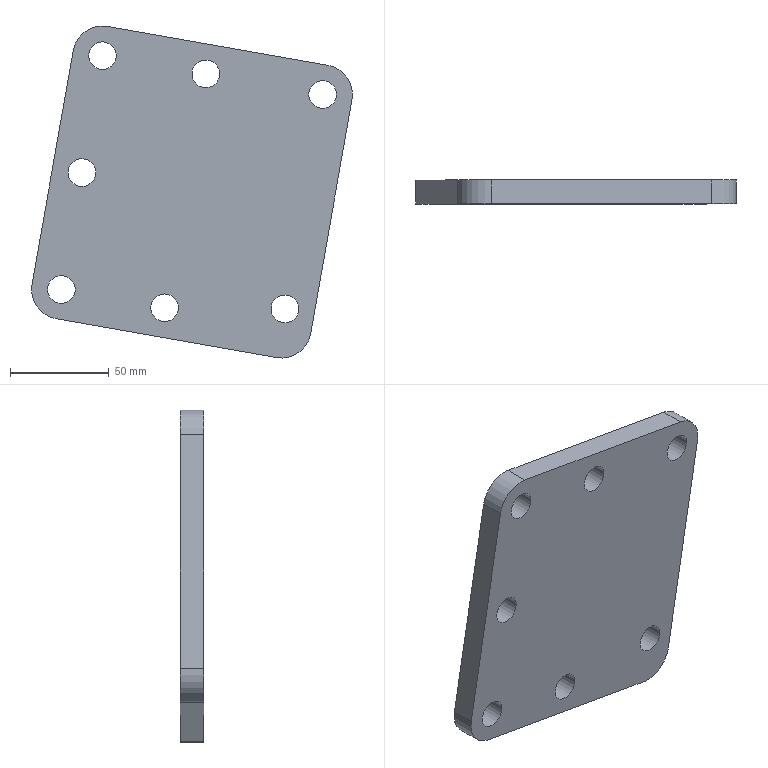Part | STEP file | front support mounting plate--000.001--20240925 | 1 solid | 17 faces | box 162.121 x 12 x 167.799 mm | volume 242152 mm3 | cylinder 11 | plane 6 | commonest cylinder face diameters 14 x7 30 x4
STEP:
#1=CARTESIAN_POINT('',(0.,0.,0.));
#2=DIRECTION('',(0.,0.,1.));
#3=DIRECTION('',(1.,0.,0.));
#4=AXIS2_PLACEMENT_3D('',#1,#2,#3);
#5=CARTESIAN_POINT('',(20.147,-188.5,-49.768));
#6=VERTEX_POINT('',#5);
#7=CARTESIAN_POINT('',(40.985,-188.5,68.409));
#8=VERTEX_POINT('',#7);
#9=CARTESIAN_POINT('',(11.873,-188.5,-96.689));
#10=DIRECTION('',(0.1736,0.,0.9848));
#11=VECTOR('',#10,1.);
#12=LINE('',#9,#11);
#13=CARTESIAN_POINT('',(30.566,-219.223,9.321));
#14=DIRECTION('',(0.9848,0.,-0.1736));
#15=DIRECTION('',(0.1736,0.,0.9848));
#16=AXIS2_PLACEMENT_3D('',#13,#14,#15);
#17=PLANE('',#16);
#18=CARTESIAN_POINT('',(-107.645,-30.723));
#19=DIRECTION('',(1.,0.));
#20=VECTOR('',#19,1.);
#21=LINE('',#18,#20);
#22=(GEOMETRIC_REPRESENTATION_CONTEXT(2)PARAMETRIC_REPRESENTATION_CONTEXT()REPRESENTATION_CONTEXT('',''));
#23=DEFINITIONAL_REPRESENTATION('',(#21),#22);
#24=PCURVE('',#17,#23);
#25=CARTESIAN_POINT('',(-243.192,-188.5,-51.714));
#26=DIRECTION('',(0.,-1.,0.));
#27=DIRECTION('',(0.1736,0.,0.9848));
#28=AXIS2_PLACEMENT_3D('',#25,#26,#27);
#29=PLANE('',#28);
#30=CARTESIAN_POINT('',(0.,-259.));
#31=DIRECTION('',(1.,0.));
#32=VECTOR('',#31,1.);
#33=LINE('',#30,#32);
#34=(GEOMETRIC_REPRESENTATION_CONTEXT(2)PARAMETRIC_REPRESENTATION_CONTEXT()REPRESENTATION_CONTEXT('',''));
#35=DEFINITIONAL_REPRESENTATION('',(#33),#34);
#36=PCURVE('',#29,#35);
#37=SURFACE_CURVE('',#12,(#24,#36),.PCURVE_S1.);
#38=EDGE_CURVE('',#6,#8,#37,.T.);
#39=ORIENTED_EDGE('',*,*,#38,.F.);
#40=CARTESIAN_POINT('',(20.147,-176.5,-49.768));
#41=VERTEX_POINT('',#40);
#42=CARTESIAN_POINT('',(20.147,-219.223,-49.768));
#43=DIRECTION('',(0.,1.,0.));
#44=VECTOR('',#43,1.);
#45=LINE('',#42,#44);
#46=CARTESIAN_POINT('',(-60.,0.));
#47=DIRECTION('',(0.,-1.));
#48=VECTOR('',#47,1.);
#49=LINE('',#46,#48);
#50=(GEOMETRIC_REPRESENTATION_CONTEXT(2)PARAMETRIC_REPRESENTATION_CONTEXT()REPRESENTATION_CONTEXT('',''));
#51=DEFINITIONAL_REPRESENTATION('',(#49),#50);
#52=PCURVE('',#17,#51);
#53=CARTESIAN_POINT('',(5.375,-188.5,-47.163));
#54=DIRECTION('',(0.,-1.,0.));
#55=DIRECTION('',(-0.2419,0.,-0.9703));
#56=AXIS2_PLACEMENT_3D('',#53,#54,#55);
#57=CYLINDRICAL_SURFACE('',#56,15.);
#58=CARTESIAN_POINT('',(1.641,30.723));
#59=DIRECTION('',(0.,-1.));
#60=VECTOR('',#59,1.);
#61=LINE('',#58,#60);
#62=(GEOMETRIC_REPRESENTATION_CONTEXT(2)PARAMETRIC_REPRESENTATION_CONTEXT()REPRESENTATION_CONTEXT('',''));
#63=DEFINITIONAL_REPRESENTATION('',(#61),#62);
#64=PCURVE('',#57,#63);
#65=SURFACE_CURVE('',#45,(#52,#64),.PCURVE_S1.);
#66=EDGE_CURVE('',#6,#41,#65,.T.);
#67=ORIENTED_EDGE('',*,*,#66,.T.);
#68=CARTESIAN_POINT('',(40.985,-176.5,68.409));
#69=VERTEX_POINT('',#68);
#70=CARTESIAN_POINT('',(11.873,-176.5,-96.689));
#71=DIRECTION('',(0.1736,0.,0.9848));
#72=VECTOR('',#71,1.);
#73=LINE('',#70,#72);
#74=CARTESIAN_POINT('',(-107.645,-42.723));
#75=DIRECTION('',(1.,0.));
#76=VECTOR('',#75,1.);
#77=LINE('',#74,#76);
#78=(GEOMETRIC_REPRESENTATION_CONTEXT(2)PARAMETRIC_REPRESENTATION_CONTEXT()REPRESENTATION_CONTEXT('',''));
#79=DEFINITIONAL_REPRESENTATION('',(#77),#78);
#80=PCURVE('',#17,#79);
#81=CARTESIAN_POINT('',(-243.192,-176.5,-51.714));
#82=DIRECTION('',(0.,-1.,0.));
#83=DIRECTION('',(0.1736,0.,0.9848));
#84=AXIS2_PLACEMENT_3D('',#81,#82,#83);
#85=PLANE('',#84);
#86=CARTESIAN_POINT('',(0.,-259.));
#87=DIRECTION('',(1.,0.));
#88=VECTOR('',#87,1.);
#89=LINE('',#86,#88);
#90=(GEOMETRIC_REPRESENTATION_CONTEXT(2)PARAMETRIC_REPRESENTATION_CONTEXT()REPRESENTATION_CONTEXT('',''));
#91=DEFINITIONAL_REPRESENTATION('',(#89),#90);
#92=PCURVE('',#85,#91);
#93=SURFACE_CURVE('',#73,(#80,#92),.PCURVE_S1.);
#94=EDGE_CURVE('',#41,#69,#93,.T.);
#95=ORIENTED_EDGE('',*,*,#94,.T.);
#96=CARTESIAN_POINT('',(40.985,-219.223,68.409));
#97=DIRECTION('',(0.,-1.,0.));
#98=VECTOR('',#97,1.);
#99=LINE('',#96,#98);
#100=CARTESIAN_POINT('',(60.,0.));
#101=DIRECTION('',(0.,1.));
#102=VECTOR('',#101,1.);
#103=LINE('',#100,#102);
#104=(GEOMETRIC_REPRESENTATION_CONTEXT(2)PARAMETRIC_REPRESENTATION_CONTEXT()REPRESENTATION_CONTEXT('',''));
#105=DEFINITIONAL_REPRESENTATION('',(#103),#104);
#106=PCURVE('',#17,#105);
#107=CARTESIAN_POINT('',(26.212,-188.5,71.014));
#108=DIRECTION('',(0.,1.,0.));
#109=DIRECTION('',(0.2419,0.,0.9703));
#110=AXIS2_PLACEMENT_3D('',#107,#108,#109);
#111=CYLINDRICAL_SURFACE('',#110,15.);
#112=CARTESIAN_POINT('',(1.501,-30.723));
#113=DIRECTION('',(0.,-1.));
#114=VECTOR('',#113,1.);
#115=LINE('',#112,#114);
#116=(GEOMETRIC_REPRESENTATION_CONTEXT(2)PARAMETRIC_REPRESENTATION_CONTEXT()REPRESENTATION_CONTEXT('',''));
#117=DEFINITIONAL_REPRESENTATION('',(#115),#116);
#118=PCURVE('',#111,#117);
#119=SURFACE_CURVE('',#99,(#106,#118),.PCURVE_S1.);
#120=EDGE_CURVE('',#69,#8,#119,.T.);
#121=ORIENTED_EDGE('',*,*,#120,.T.);
#122=EDGE_LOOP('',(#39,#67,#95,#121));
#123=FACE_BOUND('',#122,.T.);
#124=ADVANCED_FACE('',(#123),#17,.T.);
#125=CARTESIAN_POINT('',(28.817,-188.5,85.786));
#126=VERTEX_POINT('',#125);
#127=CARTESIAN_POINT('',(-82.466,-188.5,105.408));
#128=VERTEX_POINT('',#127);
#129=CARTESIAN_POINT('',(38.665,-188.5,84.049));
#130=DIRECTION('',(-0.9848,0.,0.1736));
#131=VECTOR('',#130,1.);
#132=LINE('',#129,#131);
#133=CARTESIAN_POINT('',(38.665,-188.5,84.049));
#134=DIRECTION('',(0.1736,0.,0.9848));
#135=DIRECTION('',(0.9848,0.,-0.1736));
#136=AXIS2_PLACEMENT_3D('',#133,#134,#135);
#137=PLANE('',#136);
#138=CARTESIAN_POINT('',(0.,0.));
#139=DIRECTION('',(-1.,0.));
#140=VECTOR('',#139,1.);
#141=LINE('',#138,#140);
#142=(GEOMETRIC_REPRESENTATION_CONTEXT(2)PARAMETRIC_REPRESENTATION_CONTEXT()REPRESENTATION_CONTEXT('',''));
#143=DEFINITIONAL_REPRESENTATION('',(#141),#142);
#144=PCURVE('',#137,#143);
#145=CARTESIAN_POINT('',(182.645,-254.));
#146=DIRECTION('',(0.,1.));
#147=VECTOR('',#146,1.);
#148=LINE('',#145,#147);
#149=(GEOMETRIC_REPRESENTATION_CONTEXT(2)PARAMETRIC_REPRESENTATION_CONTEXT()REPRESENTATION_CONTEXT('',''));
#150=DEFINITIONAL_REPRESENTATION('',(#148),#149);
#151=PCURVE('',#29,#150);
#152=SURFACE_CURVE('',#132,(#144,#151),.PCURVE_S1.);
#153=EDGE_CURVE('',#126,#128,#152,.T.);
#154=ORIENTED_EDGE('',*,*,#153,.F.);
#155=CARTESIAN_POINT('',(28.817,-176.5,85.786));
#156=VERTEX_POINT('',#155);
#157=CARTESIAN_POINT('',(28.817,-188.5,85.786));
#158=DIRECTION('',(0.,1.,0.));
#159=VECTOR('',#158,1.);
#160=LINE('',#157,#159);
#161=CARTESIAN_POINT('',(-10.,0.));
#162=DIRECTION('',(0.,1.));
#163=VECTOR('',#162,1.);
#164=LINE('',#161,#163);
#165=(GEOMETRIC_REPRESENTATION_CONTEXT(2)PARAMETRIC_REPRESENTATION_CONTEXT()REPRESENTATION_CONTEXT('',''));
#166=DEFINITIONAL_REPRESENTATION('',(#164),#165);
#167=PCURVE('',#137,#166);
#168=CARTESIAN_POINT('',(-0.06981,0.));
#169=DIRECTION('',(0.,1.));
#170=VECTOR('',#169,1.);
#171=LINE('',#168,#170);
#172=(GEOMETRIC_REPRESENTATION_CONTEXT(2)PARAMETRIC_REPRESENTATION_CONTEXT()REPRESENTATION_CONTEXT('',''));
#173=DEFINITIONAL_REPRESENTATION('',(#171),#172);
#174=PCURVE('',#111,#173);
#175=SURFACE_CURVE('',#160,(#167,#174),.PCURVE_S1.);
#176=EDGE_CURVE('',#126,#156,#175,.T.);
#177=ORIENTED_EDGE('',*,*,#176,.T.);
#178=CARTESIAN_POINT('',(-82.466,-176.5,105.408));
#179=VERTEX_POINT('',#178);
#180=CARTESIAN_POINT('',(-211.476,-176.5,128.156));
#181=DIRECTION('',(-0.9848,0.,0.1736));
#182=VECTOR('',#181,1.);
#183=LINE('',#180,#182);
#184=CARTESIAN_POINT('',(-254.,12.));
#185=DIRECTION('',(-1.,0.));
#186=VECTOR('',#185,1.);
#187=LINE('',#184,#186);
#188=(GEOMETRIC_REPRESENTATION_CONTEXT(2)PARAMETRIC_REPRESENTATION_CONTEXT()REPRESENTATION_CONTEXT('',''));
#189=DEFINITIONAL_REPRESENTATION('',(#187),#188);
#190=PCURVE('',#137,#189);
#191=CARTESIAN_POINT('',(182.645,0.));
#192=DIRECTION('',(0.,1.));
#193=VECTOR('',#192,1.);
#194=LINE('',#191,#193);
#195=(GEOMETRIC_REPRESENTATION_CONTEXT(2)PARAMETRIC_REPRESENTATION_CONTEXT()REPRESENTATION_CONTEXT('',''));
#196=DEFINITIONAL_REPRESENTATION('',(#194),#195);
#197=PCURVE('',#85,#196);
#198=SURFACE_CURVE('',#183,(#190,#197),.PCURVE_S1.);
#199=EDGE_CURVE('',#156,#179,#198,.T.);
#200=ORIENTED_EDGE('',*,*,#199,.T.);
#201=CARTESIAN_POINT('',(-82.466,-188.5,105.408));
#202=DIRECTION('',(0.,1.,0.));
#203=VECTOR('',#202,1.);
#204=LINE('',#201,#203);
#205=CARTESIAN_POINT('',(-123.,0.));
#206=DIRECTION('',(0.,1.));
#207=VECTOR('',#206,1.);
#208=LINE('',#205,#207);
#209=(GEOMETRIC_REPRESENTATION_CONTEXT(2)PARAMETRIC_REPRESENTATION_CONTEXT()REPRESENTATION_CONTEXT('',''));
#210=DEFINITIONAL_REPRESENTATION('',(#208),#209);
#211=PCURVE('',#137,#210);
#212=CARTESIAN_POINT('',(-85.071,-188.5,90.636));
#213=DIRECTION('',(0.,1.,0.));
#214=DIRECTION('',(0.2419,0.,0.9703));
#215=AXIS2_PLACEMENT_3D('',#212,#213,#214);
#216=CYLINDRICAL_SURFACE('',#215,15.);
#217=CARTESIAN_POINT('',(6.213,0.));
#218=DIRECTION('',(0.,1.));
#219=VECTOR('',#218,1.);
#220=LINE('',#217,#219);
#221=(GEOMETRIC_REPRESENTATION_CONTEXT(2)PARAMETRIC_REPRESENTATION_CONTEXT()REPRESENTATION_CONTEXT('',''));
#222=DEFINITIONAL_REPRESENTATION('',(#220),#221);
#223=PCURVE('',#216,#222);
#224=SURFACE_CURVE('',#204,(#211,#223),.PCURVE_S1.);
#225=EDGE_CURVE('',#128,#179,#224,.T.);
#226=ORIENTED_EDGE('',*,*,#225,.F.);
#227=EDGE_LOOP('',(#154,#177,#200,#226));
#228=FACE_BOUND('',#227,.T.);
#229=ADVANCED_FACE('',(#228),#137,.T.);
#230=CARTESIAN_POINT('',(-108.513,-176.5,-42.313));
#231=VERTEX_POINT('',#230);
#232=CARTESIAN_POINT('',(2.77,-176.5,-61.935));
#233=VERTEX_POINT('',#232);
#234=CARTESIAN_POINT('',(-237.523,-176.5,-19.565));
#235=DIRECTION('',(0.9848,0.,-0.1736));
#236=VECTOR('',#235,1.);
#237=LINE('',#234,#236);
#238=CARTESIAN_POINT('',(-108.513,-188.5,-42.313));
#239=DIRECTION('',(-0.1736,0.,-0.9848));
#240=DIRECTION('',(-0.9848,0.,0.1736));
#241=AXIS2_PLACEMENT_3D('',#238,#239,#240);
#242=PLANE('',#241);
#243=CARTESIAN_POINT('',(131.,12.));
#244=DIRECTION('',(-1.,0.));
#245=VECTOR('',#244,1.);
#246=LINE('',#243,#245);
#247=(GEOMETRIC_REPRESENTATION_CONTEXT(2)PARAMETRIC_REPRESENTATION_CONTEXT()REPRESENTATION_CONTEXT('',''));
#248=DEFINITIONAL_REPRESENTATION('',(#246),#247);
#249=PCURVE('',#242,#248);
#250=CARTESIAN_POINT('',(32.645,0.));
#251=DIRECTION('',(0.,-1.));
#252=VECTOR('',#251,1.);
#253=LINE('',#250,#252);
#254=(GEOMETRIC_REPRESENTATION_CONTEXT(2)PARAMETRIC_REPRESENTATION_CONTEXT()REPRESENTATION_CONTEXT('',''));
#255=DEFINITIONAL_REPRESENTATION('',(#253),#254);
#256=PCURVE('',#85,#255);
#257=SURFACE_CURVE('',#237,(#249,#256),.PCURVE_S1.);
#258=EDGE_CURVE('',#231,#233,#257,.T.);
#259=ORIENTED_EDGE('',*,*,#258,.T.);
#260=CARTESIAN_POINT('',(2.77,-188.5,-61.935));
#261=VERTEX_POINT('',#260);
#262=CARTESIAN_POINT('',(2.77,-188.5,-61.935));
#263=DIRECTION('',(0.,-1.,0.));
#264=VECTOR('',#263,1.);
#265=LINE('',#262,#264);
#266=CARTESIAN_POINT('',(-113.,0.));
#267=DIRECTION('',(0.,-1.));
#268=VECTOR('',#267,1.);
#269=LINE('',#266,#268);
#270=(GEOMETRIC_REPRESENTATION_CONTEXT(2)PARAMETRIC_REPRESENTATION_CONTEXT()REPRESENTATION_CONTEXT('',''));
#271=DEFINITIONAL_REPRESENTATION('',(#269),#270);
#272=PCURVE('',#242,#271);
#273=CARTESIAN_POINT('',(0.06981,0.));
#274=DIRECTION('',(0.,1.));
#275=VECTOR('',#274,1.);
#276=LINE('',#273,#275);
#277=(GEOMETRIC_REPRESENTATION_CONTEXT(2)PARAMETRIC_REPRESENTATION_CONTEXT()REPRESENTATION_CONTEXT('',''));
#278=DEFINITIONAL_REPRESENTATION('',(#276),#277);
#279=PCURVE('',#57,#278);
#280=SURFACE_CURVE('',#265,(#272,#279),.PCURVE_S1.);
#281=EDGE_CURVE('',#233,#261,#280,.T.);
#282=ORIENTED_EDGE('',*,*,#281,.T.);
#283=CARTESIAN_POINT('',(-108.513,-188.5,-42.313));
#284=VERTEX_POINT('',#283);
#285=CARTESIAN_POINT('',(-108.513,-188.5,-42.313));
#286=DIRECTION('',(0.9848,0.,-0.1736));
#287=VECTOR('',#286,1.);
#288=LINE('',#285,#287);
#289=CARTESIAN_POINT('',(0.,0.));
#290=DIRECTION('',(-1.,0.));
#291=VECTOR('',#290,1.);
#292=LINE('',#289,#291);
#293=(GEOMETRIC_REPRESENTATION_CONTEXT(2)PARAMETRIC_REPRESENTATION_CONTEXT()REPRESENTATION_CONTEXT('',''));
#294=DEFINITIONAL_REPRESENTATION('',(#292),#293);
#295=PCURVE('',#242,#294);
#296=CARTESIAN_POINT('',(32.645,-131.));
#297=DIRECTION('',(0.,-1.));
#298=VECTOR('',#297,1.);
#299=LINE('',#296,#298);
#300=(GEOMETRIC_REPRESENTATION_CONTEXT(2)PARAMETRIC_REPRESENTATION_CONTEXT()REPRESENTATION_CONTEXT('',''));
#301=DEFINITIONAL_REPRESENTATION('',(#299),#300);
#302=PCURVE('',#29,#301);
#303=SURFACE_CURVE('',#288,(#295,#302),.PCURVE_S1.);
#304=EDGE_CURVE('',#284,#261,#303,.T.);
#305=ORIENTED_EDGE('',*,*,#304,.F.);
#306=CARTESIAN_POINT('',(-108.513,-188.5,-42.313));
#307=DIRECTION('',(0.,1.,0.));
#308=VECTOR('',#307,1.);
#309=LINE('',#306,#308);
#310=CARTESIAN_POINT('',(0.,0.));
#311=DIRECTION('',(0.,1.));
#312=VECTOR('',#311,1.);
#313=LINE('',#310,#312);
#314=(GEOMETRIC_REPRESENTATION_CONTEXT(2)PARAMETRIC_REPRESENTATION_CONTEXT()REPRESENTATION_CONTEXT('',''));
#315=DEFINITIONAL_REPRESENTATION('',(#313),#314);
#316=PCURVE('',#242,#315);
#317=CARTESIAN_POINT('',(-105.909,-188.5,-27.541));
#318=DIRECTION('',(0.,1.,0.));
#319=DIRECTION('',(0.2419,0.,0.9703));
#320=AXIS2_PLACEMENT_3D('',#317,#318,#319);
#321=CYLINDRICAL_SURFACE('',#320,15.);
#322=CARTESIAN_POINT('',(3.072,0.));
#323=DIRECTION('',(0.,1.));
#324=VECTOR('',#323,1.);
#325=LINE('',#322,#324);
#326=(GEOMETRIC_REPRESENTATION_CONTEXT(2)PARAMETRIC_REPRESENTATION_CONTEXT()REPRESENTATION_CONTEXT('',''));
#327=DEFINITIONAL_REPRESENTATION('',(#325),#326);
#328=PCURVE('',#321,#327);
#329=SURFACE_CURVE('',#309,(#316,#328),.PCURVE_S1.);
#330=EDGE_CURVE('',#284,#231,#329,.T.);
#331=ORIENTED_EDGE('',*,*,#330,.T.);
#332=EDGE_LOOP('',(#259,#282,#305,#331));
#333=FACE_BOUND('',#332,.T.);
#334=ADVANCED_FACE('',(#333),#242,.T.);
#335=CARTESIAN_POINT('',(-83.377,-176.5,97.428));
#336=VERTEX_POINT('',#335);
#337=CARTESIAN_POINT('',(-85.071,-176.5,90.636));
#338=DIRECTION('',(0.,-1.,0.));
#339=DIRECTION('',(0.2419,0.,0.9703));
#340=AXIS2_PLACEMENT_3D('',#337,#338,#339);
#341=CIRCLE('',#340,7.);
#342=CARTESIAN_POINT('',(167.645,-131.));
#343=DIRECTION('',(0.9976,-0.06976));
#344=AXIS2_PLACEMENT_2D('',#342,#343);
#345=CIRCLE('',#344,7.);
#346=(GEOMETRIC_REPRESENTATION_CONTEXT(2)PARAMETRIC_REPRESENTATION_CONTEXT()REPRESENTATION_CONTEXT('',''));
#347=DEFINITIONAL_REPRESENTATION('',(#345),#346);
#348=PCURVE('',#85,#347);
#349=CARTESIAN_POINT('',(-85.071,-188.5,90.636));
#350=DIRECTION('',(0.,-1.,0.));
#351=DIRECTION('',(-0.2419,0.,-0.9703));
#352=AXIS2_PLACEMENT_3D('',#349,#350,#351);
#353=CYLINDRICAL_SURFACE('',#352,7.);
#354=CARTESIAN_POINT('',(3.142,-12.));
#355=DIRECTION('',(1.,0.));
#356=VECTOR('',#355,1.);
#357=LINE('',#354,#356);
#358=(GEOMETRIC_REPRESENTATION_CONTEXT(2)PARAMETRIC_REPRESENTATION_CONTEXT()REPRESENTATION_CONTEXT('',''));
#359=DEFINITIONAL_REPRESENTATION('',(#357),#358);
#360=PCURVE('',#353,#359);
#361=SURFACE_CURVE('',#341,(#348,#360),.PCURVE_S1.);
#362=EDGE_CURVE('',#336,#336,#361,.T.);
#363=ORIENTED_EDGE('',*,*,#362,.T.);
#364=EDGE_LOOP('',(#363));
#365=FACE_BOUND('',#364,.T.);
#366=CARTESIAN_POINT('',(-31.183,-176.5,88.225));
#367=VERTEX_POINT('',#366);
#368=CARTESIAN_POINT('',(-32.876,-176.5,81.433));
#369=DIRECTION('',(0.,-1.,0.));
#370=DIRECTION('',(0.2419,0.,0.9703));
#371=AXIS2_PLACEMENT_3D('',#368,#369,#370);
#372=CIRCLE('',#371,7.);
#373=CARTESIAN_POINT('',(167.645,-184.));
#374=DIRECTION('',(0.9976,-0.06976));
#375=AXIS2_PLACEMENT_2D('',#373,#374);
#376=CIRCLE('',#375,7.);
#377=(GEOMETRIC_REPRESENTATION_CONTEXT(2)PARAMETRIC_REPRESENTATION_CONTEXT()REPRESENTATION_CONTEXT('',''));
#378=DEFINITIONAL_REPRESENTATION('',(#376),#377);
#379=PCURVE('',#85,#378);
#380=CARTESIAN_POINT('',(-32.876,-188.5,81.433));
#381=DIRECTION('',(0.,-1.,0.));
#382=DIRECTION('',(-0.2419,0.,-0.9703));
#383=AXIS2_PLACEMENT_3D('',#380,#381,#382);
#384=CYLINDRICAL_SURFACE('',#383,7.);
#385=CARTESIAN_POINT('',(3.142,-12.));
#386=DIRECTION('',(1.,0.));
#387=VECTOR('',#386,1.);
#388=LINE('',#385,#387);
#389=(GEOMETRIC_REPRESENTATION_CONTEXT(2)PARAMETRIC_REPRESENTATION_CONTEXT()REPRESENTATION_CONTEXT('',''));
#390=DEFINITIONAL_REPRESENTATION('',(#388),#389);
#391=PCURVE('',#384,#390);
#392=SURFACE_CURVE('',#372,(#379,#391),.PCURVE_S1.);
#393=EDGE_CURVE('',#367,#367,#392,.T.);
#394=ORIENTED_EDGE('',*,*,#393,.T.);
#395=EDGE_LOOP('',(#394));
#396=FACE_BOUND('',#395,.T.);
#397=CARTESIAN_POINT('',(27.906,-176.5,77.806));
#398=VERTEX_POINT('',#397);
#399=CARTESIAN_POINT('',(26.212,-176.5,71.014));
#400=DIRECTION('',(0.,-1.,0.));
#401=DIRECTION('',(0.2419,0.,0.9703));
#402=AXIS2_PLACEMENT_3D('',#399,#400,#401);
#403=CIRCLE('',#402,7.);
#404=CARTESIAN_POINT('',(167.645,-244.));
#405=DIRECTION('',(0.9976,-0.06976));
#406=AXIS2_PLACEMENT_2D('',#404,#405);
#407=CIRCLE('',#406,7.);
#408=(GEOMETRIC_REPRESENTATION_CONTEXT(2)PARAMETRIC_REPRESENTATION_CONTEXT()REPRESENTATION_CONTEXT('',''));
#409=DEFINITIONAL_REPRESENTATION('',(#407),#408);
#410=PCURVE('',#85,#409);
#411=CARTESIAN_POINT('',(26.212,-188.5,71.014));
#412=DIRECTION('',(0.,-1.,0.));
#413=DIRECTION('',(-0.2419,0.,-0.9703));
#414=AXIS2_PLACEMENT_3D('',#411,#412,#413);
#415=CYLINDRICAL_SURFACE('',#414,7.);
#416=CARTESIAN_POINT('',(3.142,-12.));
#417=DIRECTION('',(1.,0.));
#418=VECTOR('',#417,1.);
#419=LINE('',#416,#418);
#420=(GEOMETRIC_REPRESENTATION_CONTEXT(2)PARAMETRIC_REPRESENTATION_CONTEXT()REPRESENTATION_CONTEXT('',''));
#421=DEFINITIONAL_REPRESENTATION('',(#419),#420);
#422=PCURVE('',#415,#421);
#423=SURFACE_CURVE('',#403,(#410,#422),.PCURVE_S1.);
#424=EDGE_CURVE('',#398,#398,#423,.T.);
#425=ORIENTED_EDGE('',*,*,#424,.T.);
#426=EDGE_LOOP('',(#425));
#427=FACE_BOUND('',#426,.T.);
#428=CARTESIAN_POINT('',(-93.796,-176.5,38.34));
#429=VERTEX_POINT('',#428);
#430=CARTESIAN_POINT('',(-95.49,-176.5,31.548));
#431=DIRECTION('',(0.,-1.,0.));
#432=DIRECTION('',(0.2419,0.,0.9703));
#433=AXIS2_PLACEMENT_3D('',#430,#431,#432);
#434=CIRCLE('',#433,7.);
#435=CARTESIAN_POINT('',(107.645,-131.));
#436=DIRECTION('',(0.9976,-0.06976));
#437=AXIS2_PLACEMENT_2D('',#435,#436);
#438=CIRCLE('',#437,7.);
#439=(GEOMETRIC_REPRESENTATION_CONTEXT(2)PARAMETRIC_REPRESENTATION_CONTEXT()REPRESENTATION_CONTEXT('',''));
#440=DEFINITIONAL_REPRESENTATION('',(#438),#439);
#441=PCURVE('',#85,#440);
#442=CARTESIAN_POINT('',(-95.49,-188.5,31.548));
#443=DIRECTION('',(0.,-1.,0.));
#444=DIRECTION('',(-0.2419,0.,-0.9703));
#445=AXIS2_PLACEMENT_3D('',#442,#443,#444);
#446=CYLINDRICAL_SURFACE('',#445,7.);
#447=CARTESIAN_POINT('',(3.142,-12.));
#448=DIRECTION('',(1.,0.));
#449=VECTOR('',#448,1.);
#450=LINE('',#447,#449);
#451=(GEOMETRIC_REPRESENTATION_CONTEXT(2)PARAMETRIC_REPRESENTATION_CONTEXT()REPRESENTATION_CONTEXT('',''));
#452=DEFINITIONAL_REPRESENTATION('',(#450),#451);
#453=PCURVE('',#446,#452);
#454=SURFACE_CURVE('',#434,(#441,#453),.PCURVE_S1.);
#455=EDGE_CURVE('',#429,#429,#454,.T.);
#456=ORIENTED_EDGE('',*,*,#455,.T.);
#457=EDGE_LOOP('',(#456));
#458=FACE_BOUND('',#457,.T.);
#459=CARTESIAN_POINT('',(8.805,-176.5,-30.523));
#460=VERTEX_POINT('',#459);
#461=CARTESIAN_POINT('',(7.111,-176.5,-37.315));
#462=DIRECTION('',(0.,-1.,0.));
#463=DIRECTION('',(0.2419,0.,0.9703));
#464=AXIS2_PLACEMENT_3D('',#461,#462,#463);
#465=CIRCLE('',#464,7.);
#466=CARTESIAN_POINT('',(57.645,-244.));
#467=DIRECTION('',(0.9976,-0.06976));
#468=AXIS2_PLACEMENT_2D('',#466,#467);
#469=CIRCLE('',#468,7.);
#470=(GEOMETRIC_REPRESENTATION_CONTEXT(2)PARAMETRIC_REPRESENTATION_CONTEXT()REPRESENTATION_CONTEXT('',''));
#471=DEFINITIONAL_REPRESENTATION('',(#469),#470);
#472=PCURVE('',#85,#471);
#473=CARTESIAN_POINT('',(7.111,-188.5,-37.315));
#474=DIRECTION('',(0.,-1.,0.));
#475=DIRECTION('',(-0.2419,0.,-0.9703));
#476=AXIS2_PLACEMENT_3D('',#473,#474,#475);
#477=CYLINDRICAL_SURFACE('',#476,7.);
#478=CARTESIAN_POINT('',(3.142,-12.));
#479=DIRECTION('',(1.,0.));
#480=VECTOR('',#479,1.);
#481=LINE('',#478,#480);
#482=(GEOMETRIC_REPRESENTATION_CONTEXT(2)PARAMETRIC_REPRESENTATION_CONTEXT()REPRESENTATION_CONTEXT('',''));
#483=DEFINITIONAL_REPRESENTATION('',(#481),#482);
#484=PCURVE('',#477,#483);
#485=SURFACE_CURVE('',#465,(#472,#484),.PCURVE_S1.);
#486=EDGE_CURVE('',#460,#460,#485,.T.);
#487=ORIENTED_EDGE('',*,*,#486,.T.);
#488=EDGE_LOOP('',(#487));
#489=FACE_BOUND('',#488,.T.);
#490=CARTESIAN_POINT('',(-104.215,-176.5,-20.749));
#491=VERTEX_POINT('',#490);
#492=CARTESIAN_POINT('',(-105.909,-176.5,-27.541));
#493=DIRECTION('',(0.,-1.,0.));
#494=DIRECTION('',(0.2419,0.,0.9703));
#495=AXIS2_PLACEMENT_3D('',#492,#493,#494);
#496=CIRCLE('',#495,7.);
#497=CARTESIAN_POINT('',(47.645,-131.));
#498=DIRECTION('',(0.9976,-0.06976));
#499=AXIS2_PLACEMENT_2D('',#497,#498);
#500=CIRCLE('',#499,7.);
#501=(GEOMETRIC_REPRESENTATION_CONTEXT(2)PARAMETRIC_REPRESENTATION_CONTEXT()REPRESENTATION_CONTEXT('',''));
#502=DEFINITIONAL_REPRESENTATION('',(#500),#501);
#503=PCURVE('',#85,#502);
#504=CARTESIAN_POINT('',(-105.909,-188.5,-27.541));
#505=DIRECTION('',(0.,-1.,0.));
#506=DIRECTION('',(-0.2419,0.,-0.9703));
#507=AXIS2_PLACEMENT_3D('',#504,#505,#506);
#508=CYLINDRICAL_SURFACE('',#507,7.);
#509=CARTESIAN_POINT('',(3.142,-12.));
#510=DIRECTION('',(1.,0.));
#511=VECTOR('',#510,1.);
#512=LINE('',#509,#511);
#513=(GEOMETRIC_REPRESENTATION_CONTEXT(2)PARAMETRIC_REPRESENTATION_CONTEXT()REPRESENTATION_CONTEXT('',''));
#514=DEFINITIONAL_REPRESENTATION('',(#512),#513);
#515=PCURVE('',#508,#514);
#516=SURFACE_CURVE('',#496,(#503,#515),.PCURVE_S1.);
#517=EDGE_CURVE('',#491,#491,#516,.T.);
#518=ORIENTED_EDGE('',*,*,#517,.T.);
#519=EDGE_LOOP('',(#518));
#520=FACE_BOUND('',#519,.T.);
#521=CARTESIAN_POINT('',(-52.02,-176.5,-29.952));
#522=VERTEX_POINT('',#521);
#523=CARTESIAN_POINT('',(-53.714,-176.5,-36.744));
#524=DIRECTION('',(0.,-1.,0.));
#525=DIRECTION('',(0.2419,0.,0.9703));
#526=AXIS2_PLACEMENT_3D('',#523,#524,#525);
#527=CIRCLE('',#526,7.);
#528=CARTESIAN_POINT('',(47.645,-184.));
#529=DIRECTION('',(0.9976,-0.06976));
#530=AXIS2_PLACEMENT_2D('',#528,#529);
#531=CIRCLE('',#530,7.);
#532=(GEOMETRIC_REPRESENTATION_CONTEXT(2)PARAMETRIC_REPRESENTATION_CONTEXT()REPRESENTATION_CONTEXT('',''));
#533=DEFINITIONAL_REPRESENTATION('',(#531),#532);
#534=PCURVE('',#85,#533);
#535=CARTESIAN_POINT('',(-53.714,-188.5,-36.744));
#536=DIRECTION('',(0.,-1.,0.));
#537=DIRECTION('',(-0.2419,0.,-0.9703));
#538=AXIS2_PLACEMENT_3D('',#535,#536,#537);
#539=CYLINDRICAL_SURFACE('',#538,7.);
#540=CARTESIAN_POINT('',(3.142,-12.));
#541=DIRECTION('',(1.,0.));
#542=VECTOR('',#541,1.);
#543=LINE('',#540,#542);
#544=(GEOMETRIC_REPRESENTATION_CONTEXT(2)PARAMETRIC_REPRESENTATION_CONTEXT()REPRESENTATION_CONTEXT('',''));
#545=DEFINITIONAL_REPRESENTATION('',(#543),#544);
#546=PCURVE('',#539,#545);
#547=SURFACE_CURVE('',#527,(#534,#546),.PCURVE_S1.);
#548=EDGE_CURVE('',#522,#522,#547,.T.);
#549=ORIENTED_EDGE('',*,*,#548,.T.);
#550=EDGE_LOOP('',(#549));
#551=FACE_BOUND('',#550,.T.);
#552=ORIENTED_EDGE('',*,*,#94,.F.);
#553=CARTESIAN_POINT('',(5.375,-176.5,-47.163));
#554=DIRECTION('',(0.,1.,0.));
#555=DIRECTION('',(0.2419,0.,0.9703));
#556=AXIS2_PLACEMENT_3D('',#553,#554,#555);
#557=CIRCLE('',#556,15.);
#558=CARTESIAN_POINT('',(62.608,-245.046));
#559=CARTESIAN_POINT('',(60.796,-270.964));
#560=CARTESIAN_POINT('',(39.257,-256.436));
#561=CARTESIAN_POINT('',(17.718,-241.907));
#562=CARTESIAN_POINT('',(41.069,-230.518));
#563=CARTESIAN_POINT('',(64.42,-219.129));
#564=CARTESIAN_POINT('',(62.608,-245.046));
#565=(BOUNDED_CURVE()B_SPLINE_CURVE(2,(#558,#559,#560,#561,#562,#563,#564),.UNSPECIFIED.,.T.,.F.)B_SPLINE_CURVE_WITH_KNOTS((1,2,2,2,2,1),(-2.094,0.,2.094,4.189,6.283,8.378),.UNSPECIFIED.)CURVE()GEOMETRIC_REPRESENTATION_ITEM()RATIONAL_B_SPLINE_CURVE((1.,0.5,1.,0.5,1.,0.5,1.))REPRESENTATION_ITEM(''));
#566=(GEOMETRIC_REPRESENTATION_CONTEXT(2)PARAMETRIC_REPRESENTATION_CONTEXT()REPRESENTATION_CONTEXT('',''));
#567=DEFINITIONAL_REPRESENTATION('',(#565),#566);
#568=PCURVE('',#85,#567);
#569=CARTESIAN_POINT('',(3.142,-12.));
#570=DIRECTION('',(-1.,0.));
#571=VECTOR('',#570,1.);
#572=LINE('',#569,#571);
#573=(GEOMETRIC_REPRESENTATION_CONTEXT(2)PARAMETRIC_REPRESENTATION_CONTEXT()REPRESENTATION_CONTEXT('',''));
#574=DEFINITIONAL_REPRESENTATION('',(#572),#573);
#575=PCURVE('',#57,#574);
#576=SURFACE_CURVE('',#557,(#568,#575),.PCURVE_S1.);
#577=EDGE_CURVE('',#41,#233,#576,.T.);
#578=ORIENTED_EDGE('',*,*,#577,.T.);
#579=ORIENTED_EDGE('',*,*,#258,.F.);
#580=CARTESIAN_POINT('',(-120.681,-176.5,-24.936));
#581=VERTEX_POINT('',#580);
#582=CARTESIAN_POINT('',(-105.909,-176.5,-27.541));
#583=DIRECTION('',(0.,1.,0.));
#584=DIRECTION('',(-0.2419,0.,-0.9703));
#585=AXIS2_PLACEMENT_3D('',#582,#583,#584);
#586=CIRCLE('',#585,15.);
#587=CARTESIAN_POINT('',(32.681,-129.954));
#588=CARTESIAN_POINT('',(34.494,-104.036));
#589=CARTESIAN_POINT('',(56.033,-118.564));
#590=CARTESIAN_POINT('',(77.572,-133.093));
#591=CARTESIAN_POINT('',(54.22,-144.482));
#592=CARTESIAN_POINT('',(30.869,-155.871));
#593=CARTESIAN_POINT('',(32.681,-129.954));
#594=(BOUNDED_CURVE()B_SPLINE_CURVE(2,(#587,#588,#589,#590,#591,#592,#593),.UNSPECIFIED.,.T.,.F.)B_SPLINE_CURVE_WITH_KNOTS((1,2,2,2,2,1),(-2.094,0.,2.094,4.189,6.283,8.378),.UNSPECIFIED.)CURVE()GEOMETRIC_REPRESENTATION_ITEM()RATIONAL_B_SPLINE_CURVE((1.,0.5,1.,0.5,1.,0.5,1.))REPRESENTATION_ITEM(''));
#595=(GEOMETRIC_REPRESENTATION_CONTEXT(2)PARAMETRIC_REPRESENTATION_CONTEXT()REPRESENTATION_CONTEXT('',''));
#596=DEFINITIONAL_REPRESENTATION('',(#594),#595);
#597=PCURVE('',#85,#596);
#598=CARTESIAN_POINT('',(-3.142,12.));
#599=DIRECTION('',(1.,0.));
#600=VECTOR('',#599,1.);
#601=LINE('',#598,#600);
#602=(GEOMETRIC_REPRESENTATION_CONTEXT(2)PARAMETRIC_REPRESENTATION_CONTEXT()REPRESENTATION_CONTEXT('',''));
#603=DEFINITIONAL_REPRESENTATION('',(#601),#602);
#604=PCURVE('',#321,#603);
#605=SURFACE_CURVE('',#586,(#597,#604),.PCURVE_S1.);
#606=EDGE_CURVE('',#231,#581,#605,.T.);
#607=ORIENTED_EDGE('',*,*,#606,.T.);
#608=CARTESIAN_POINT('',(-99.843,-176.5,93.241));
#609=VERTEX_POINT('',#608);
#610=CARTESIAN_POINT('',(-128.954,-176.5,-71.857));
#611=DIRECTION('',(-0.1736,0.,-0.9848));
#612=VECTOR('',#611,1.);
#613=LINE('',#610,#612);
#614=CARTESIAN_POINT('',(0.,-116.));
#615=DIRECTION('',(-1.,0.));
#616=VECTOR('',#615,1.);
#617=LINE('',#614,#616);
#618=(GEOMETRIC_REPRESENTATION_CONTEXT(2)PARAMETRIC_REPRESENTATION_CONTEXT()REPRESENTATION_CONTEXT('',''));
#619=DEFINITIONAL_REPRESENTATION('',(#617),#618);
#620=PCURVE('',#85,#619);
#621=CARTESIAN_POINT('',(-99.843,-188.5,93.241));
#622=DIRECTION('',(-0.9848,0.,0.1736));
#623=DIRECTION('',(0.1736,0.,0.9848));
#624=AXIS2_PLACEMENT_3D('',#621,#622,#623);
#625=PLANE('',#624);
#626=CARTESIAN_POINT('',(-167.645,12.));
#627=DIRECTION('',(-1.,0.));
#628=VECTOR('',#627,1.);
#629=LINE('',#626,#628);
#630=(GEOMETRIC_REPRESENTATION_CONTEXT(2)PARAMETRIC_REPRESENTATION_CONTEXT()REPRESENTATION_CONTEXT('',''));
#631=DEFINITIONAL_REPRESENTATION('',(#629),#630);
#632=PCURVE('',#625,#631);
#633=SURFACE_CURVE('',#613,(#620,#632),.PCURVE_S1.);
#634=EDGE_CURVE('',#609,#581,#633,.T.);
#635=ORIENTED_EDGE('',*,*,#634,.F.);
#636=CARTESIAN_POINT('',(-85.071,-176.5,90.636));
#637=DIRECTION('',(0.,1.,0.));
#638=DIRECTION('',(-0.2419,0.,-0.9703));
#639=AXIS2_PLACEMENT_3D('',#636,#637,#638);
#640=CIRCLE('',#639,15.);
#641=CARTESIAN_POINT('',(152.681,-129.954));
#642=CARTESIAN_POINT('',(154.494,-104.036));
#643=CARTESIAN_POINT('',(176.033,-118.564));
#644=CARTESIAN_POINT('',(197.572,-133.093));
#645=CARTESIAN_POINT('',(174.22,-144.482));
#646=CARTESIAN_POINT('',(150.869,-155.871));
#647=CARTESIAN_POINT('',(152.681,-129.954));
#648=(BOUNDED_CURVE()B_SPLINE_CURVE(2,(#641,#642,#643,#644,#645,#646,#647),.UNSPECIFIED.,.T.,.F.)B_SPLINE_CURVE_WITH_KNOTS((1,2,2,2,2,1),(-2.094,0.,2.094,4.189,6.283,8.378),.UNSPECIFIED.)CURVE()GEOMETRIC_REPRESENTATION_ITEM()RATIONAL_B_SPLINE_CURVE((1.,0.5,1.,0.5,1.,0.5,1.))REPRESENTATION_ITEM(''));
#649=(GEOMETRIC_REPRESENTATION_CONTEXT(2)PARAMETRIC_REPRESENTATION_CONTEXT()REPRESENTATION_CONTEXT('',''));
#650=DEFINITIONAL_REPRESENTATION('',(#648),#649);
#651=PCURVE('',#85,#650);
#652=CARTESIAN_POINT('',(3.142,12.));
#653=DIRECTION('',(1.,0.));
#654=VECTOR('',#653,1.);
#655=LINE('',#652,#654);
#656=(GEOMETRIC_REPRESENTATION_CONTEXT(2)PARAMETRIC_REPRESENTATION_CONTEXT()REPRESENTATION_CONTEXT('',''));
#657=DEFINITIONAL_REPRESENTATION('',(#655),#656);
#658=PCURVE('',#216,#657);
#659=SURFACE_CURVE('',#640,(#651,#658),.PCURVE_S1.);
#660=EDGE_CURVE('',#609,#179,#659,.T.);
#661=ORIENTED_EDGE('',*,*,#660,.T.);
#662=ORIENTED_EDGE('',*,*,#199,.F.);
#663=CARTESIAN_POINT('',(26.212,-176.5,71.014));
#664=DIRECTION('',(0.,1.,0.));
#665=DIRECTION('',(0.2419,0.,0.9703));
#666=AXIS2_PLACEMENT_3D('',#663,#664,#665);
#667=CIRCLE('',#666,15.);
#668=CARTESIAN_POINT('',(182.608,-245.046));
#669=CARTESIAN_POINT('',(180.796,-270.964));
#670=CARTESIAN_POINT('',(159.257,-256.436));
#671=CARTESIAN_POINT('',(137.718,-241.907));
#672=CARTESIAN_POINT('',(161.069,-230.518));
#673=CARTESIAN_POINT('',(184.42,-219.129));
#674=CARTESIAN_POINT('',(182.608,-245.046));
#675=(BOUNDED_CURVE()B_SPLINE_CURVE(2,(#668,#669,#670,#671,#672,#673,#674),.UNSPECIFIED.,.T.,.F.)B_SPLINE_CURVE_WITH_KNOTS((1,2,2,2,2,1),(-2.094,0.,2.094,4.189,6.283,8.378),.UNSPECIFIED.)CURVE()GEOMETRIC_REPRESENTATION_ITEM()RATIONAL_B_SPLINE_CURVE((1.,0.5,1.,0.5,1.,0.5,1.))REPRESENTATION_ITEM(''));
#676=(GEOMETRIC_REPRESENTATION_CONTEXT(2)PARAMETRIC_REPRESENTATION_CONTEXT()REPRESENTATION_CONTEXT('',''));
#677=DEFINITIONAL_REPRESENTATION('',(#675),#676);
#678=PCURVE('',#85,#677);
#679=CARTESIAN_POINT('',(-6.283,12.));
#680=DIRECTION('',(1.,0.));
#681=VECTOR('',#680,1.);
#682=LINE('',#679,#681);
#683=(GEOMETRIC_REPRESENTATION_CONTEXT(2)PARAMETRIC_REPRESENTATION_CONTEXT()REPRESENTATION_CONTEXT('',''));
#684=DEFINITIONAL_REPRESENTATION('',(#682),#683);
#685=PCURVE('',#111,#684);
#686=SURFACE_CURVE('',#667,(#678,#685),.PCURVE_S1.);
#687=EDGE_CURVE('',#156,#69,#686,.T.);
#688=ORIENTED_EDGE('',*,*,#687,.T.);
#689=EDGE_LOOP('',(#552,#578,#579,#607,#635,#661,#662,#688));
#690=FACE_BOUND('',#689,.T.);
#691=ADVANCED_FACE('',(#365,#396,#427,#458,#489,#520,#551,#690),#85,.F.);
#692=CARTESIAN_POINT('',(-52.02,-188.5,-29.952));
#693=VERTEX_POINT('',#692);
#694=CARTESIAN_POINT('',(-53.714,-188.5,-36.744));
#695=DIRECTION('',(0.,-1.,0.));
#696=DIRECTION('',(0.2419,0.,0.9703));
#697=AXIS2_PLACEMENT_3D('',#694,#695,#696);
#698=CIRCLE('',#697,7.);
#699=CARTESIAN_POINT('',(47.645,-184.));
#700=DIRECTION('',(0.9976,-0.06976));
#701=AXIS2_PLACEMENT_2D('',#699,#700);
#702=CIRCLE('',#701,7.);
#703=(GEOMETRIC_REPRESENTATION_CONTEXT(2)PARAMETRIC_REPRESENTATION_CONTEXT()REPRESENTATION_CONTEXT('',''));
#704=DEFINITIONAL_REPRESENTATION('',(#702),#703);
#705=PCURVE('',#29,#704);
#706=CARTESIAN_POINT('',(3.142,0.));
#707=DIRECTION('',(1.,0.));
#708=VECTOR('',#707,1.);
#709=LINE('',#706,#708);
#710=(GEOMETRIC_REPRESENTATION_CONTEXT(2)PARAMETRIC_REPRESENTATION_CONTEXT()REPRESENTATION_CONTEXT('',''));
#711=DEFINITIONAL_REPRESENTATION('',(#709),#710);
#712=PCURVE('',#539,#711);
#713=SURFACE_CURVE('',#698,(#705,#712),.PCURVE_S1.);
#714=EDGE_CURVE('',#693,#693,#713,.T.);
#715=ORIENTED_EDGE('',*,*,#714,.F.);
#716=EDGE_LOOP('',(#715));
#717=FACE_BOUND('',#716,.T.);
#718=CARTESIAN_POINT('',(-104.215,-188.5,-20.749));
#719=VERTEX_POINT('',#718);
#720=CARTESIAN_POINT('',(-105.909,-188.5,-27.541));
#721=DIRECTION('',(0.,-1.,0.));
#722=DIRECTION('',(0.2419,0.,0.9703));
#723=AXIS2_PLACEMENT_3D('',#720,#721,#722);
#724=CIRCLE('',#723,7.);
#725=CARTESIAN_POINT('',(47.645,-131.));
#726=DIRECTION('',(0.9976,-0.06976));
#727=AXIS2_PLACEMENT_2D('',#725,#726);
#728=CIRCLE('',#727,7.);
#729=(GEOMETRIC_REPRESENTATION_CONTEXT(2)PARAMETRIC_REPRESENTATION_CONTEXT()REPRESENTATION_CONTEXT('',''));
#730=DEFINITIONAL_REPRESENTATION('',(#728),#729);
#731=PCURVE('',#29,#730);
#732=CARTESIAN_POINT('',(3.142,0.));
#733=DIRECTION('',(1.,0.));
#734=VECTOR('',#733,1.);
#735=LINE('',#732,#734);
#736=(GEOMETRIC_REPRESENTATION_CONTEXT(2)PARAMETRIC_REPRESENTATION_CONTEXT()REPRESENTATION_CONTEXT('',''));
#737=DEFINITIONAL_REPRESENTATION('',(#735),#736);
#738=PCURVE('',#508,#737);
#739=SURFACE_CURVE('',#724,(#731,#738),.PCURVE_S1.);
#740=EDGE_CURVE('',#719,#719,#739,.T.);
#741=ORIENTED_EDGE('',*,*,#740,.F.);
#742=EDGE_LOOP('',(#741));
#743=FACE_BOUND('',#742,.T.);
#744=CARTESIAN_POINT('',(8.805,-188.5,-30.523));
#745=VERTEX_POINT('',#744);
#746=CARTESIAN_POINT('',(7.111,-188.5,-37.315));
#747=DIRECTION('',(0.,-1.,0.));
#748=DIRECTION('',(0.2419,0.,0.9703));
#749=AXIS2_PLACEMENT_3D('',#746,#747,#748);
#750=CIRCLE('',#749,7.);
#751=CARTESIAN_POINT('',(57.645,-244.));
#752=DIRECTION('',(0.9976,-0.06976));
#753=AXIS2_PLACEMENT_2D('',#751,#752);
#754=CIRCLE('',#753,7.);
#755=(GEOMETRIC_REPRESENTATION_CONTEXT(2)PARAMETRIC_REPRESENTATION_CONTEXT()REPRESENTATION_CONTEXT('',''));
#756=DEFINITIONAL_REPRESENTATION('',(#754),#755);
#757=PCURVE('',#29,#756);
#758=CARTESIAN_POINT('',(3.142,0.));
#759=DIRECTION('',(1.,0.));
#760=VECTOR('',#759,1.);
#761=LINE('',#758,#760);
#762=(GEOMETRIC_REPRESENTATION_CONTEXT(2)PARAMETRIC_REPRESENTATION_CONTEXT()REPRESENTATION_CONTEXT('',''));
#763=DEFINITIONAL_REPRESENTATION('',(#761),#762);
#764=PCURVE('',#477,#763);
#765=SURFACE_CURVE('',#750,(#757,#764),.PCURVE_S1.);
#766=EDGE_CURVE('',#745,#745,#765,.T.);
#767=ORIENTED_EDGE('',*,*,#766,.F.);
#768=EDGE_LOOP('',(#767));
#769=FACE_BOUND('',#768,.T.);
#770=CARTESIAN_POINT('',(-93.796,-188.5,38.34));
#771=VERTEX_POINT('',#770);
#772=CARTESIAN_POINT('',(-95.49,-188.5,31.548));
#773=DIRECTION('',(0.,-1.,0.));
#774=DIRECTION('',(0.2419,0.,0.9703));
#775=AXIS2_PLACEMENT_3D('',#772,#773,#774);
#776=CIRCLE('',#775,7.);
#777=CARTESIAN_POINT('',(107.645,-131.));
#778=DIRECTION('',(0.9976,-0.06976));
#779=AXIS2_PLACEMENT_2D('',#777,#778);
#780=CIRCLE('',#779,7.);
#781=(GEOMETRIC_REPRESENTATION_CONTEXT(2)PARAMETRIC_REPRESENTATION_CONTEXT()REPRESENTATION_CONTEXT('',''));
#782=DEFINITIONAL_REPRESENTATION('',(#780),#781);
#783=PCURVE('',#29,#782);
#784=CARTESIAN_POINT('',(3.142,0.));
#785=DIRECTION('',(1.,0.));
#786=VECTOR('',#785,1.);
#787=LINE('',#784,#786);
#788=(GEOMETRIC_REPRESENTATION_CONTEXT(2)PARAMETRIC_REPRESENTATION_CONTEXT()REPRESENTATION_CONTEXT('',''));
#789=DEFINITIONAL_REPRESENTATION('',(#787),#788);
#790=PCURVE('',#446,#789);
#791=SURFACE_CURVE('',#776,(#783,#790),.PCURVE_S1.);
#792=EDGE_CURVE('',#771,#771,#791,.T.);
#793=ORIENTED_EDGE('',*,*,#792,.F.);
#794=EDGE_LOOP('',(#793));
#795=FACE_BOUND('',#794,.T.);
#796=CARTESIAN_POINT('',(27.906,-188.5,77.806));
#797=VERTEX_POINT('',#796);
#798=CARTESIAN_POINT('',(26.212,-188.5,71.014));
#799=DIRECTION('',(0.,-1.,0.));
#800=DIRECTION('',(0.2419,0.,0.9703));
#801=AXIS2_PLACEMENT_3D('',#798,#799,#800);
#802=CIRCLE('',#801,7.);
#803=CARTESIAN_POINT('',(167.645,-244.));
#804=DIRECTION('',(0.9976,-0.06976));
#805=AXIS2_PLACEMENT_2D('',#803,#804);
#806=CIRCLE('',#805,7.);
#807=(GEOMETRIC_REPRESENTATION_CONTEXT(2)PARAMETRIC_REPRESENTATION_CONTEXT()REPRESENTATION_CONTEXT('',''));
#808=DEFINITIONAL_REPRESENTATION('',(#806),#807);
#809=PCURVE('',#29,#808);
#810=CARTESIAN_POINT('',(3.142,0.));
#811=DIRECTION('',(1.,0.));
#812=VECTOR('',#811,1.);
#813=LINE('',#810,#812);
#814=(GEOMETRIC_REPRESENTATION_CONTEXT(2)PARAMETRIC_REPRESENTATION_CONTEXT()REPRESENTATION_CONTEXT('',''));
#815=DEFINITIONAL_REPRESENTATION('',(#813),#814);
#816=PCURVE('',#415,#815);
#817=SURFACE_CURVE('',#802,(#809,#816),.PCURVE_S1.);
#818=EDGE_CURVE('',#797,#797,#817,.T.);
#819=ORIENTED_EDGE('',*,*,#818,.F.);
#820=EDGE_LOOP('',(#819));
#821=FACE_BOUND('',#820,.T.);
#822=CARTESIAN_POINT('',(-31.183,-188.5,88.225));
#823=VERTEX_POINT('',#822);
#824=CARTESIAN_POINT('',(-32.876,-188.5,81.433));
#825=DIRECTION('',(0.,-1.,0.));
#826=DIRECTION('',(0.2419,0.,0.9703));
#827=AXIS2_PLACEMENT_3D('',#824,#825,#826);
#828=CIRCLE('',#827,7.);
#829=CARTESIAN_POINT('',(167.645,-184.));
#830=DIRECTION('',(0.9976,-0.06976));
#831=AXIS2_PLACEMENT_2D('',#829,#830);
#832=CIRCLE('',#831,7.);
#833=(GEOMETRIC_REPRESENTATION_CONTEXT(2)PARAMETRIC_REPRESENTATION_CONTEXT()REPRESENTATION_CONTEXT('',''));
#834=DEFINITIONAL_REPRESENTATION('',(#832),#833);
#835=PCURVE('',#29,#834);
#836=CARTESIAN_POINT('',(3.142,0.));
#837=DIRECTION('',(1.,0.));
#838=VECTOR('',#837,1.);
#839=LINE('',#836,#838);
#840=(GEOMETRIC_REPRESENTATION_CONTEXT(2)PARAMETRIC_REPRESENTATION_CONTEXT()REPRESENTATION_CONTEXT('',''));
#841=DEFINITIONAL_REPRESENTATION('',(#839),#840);
#842=PCURVE('',#384,#841);
#843=SURFACE_CURVE('',#828,(#835,#842),.PCURVE_S1.);
#844=EDGE_CURVE('',#823,#823,#843,.T.);
#845=ORIENTED_EDGE('',*,*,#844,.F.);
#846=EDGE_LOOP('',(#845));
#847=FACE_BOUND('',#846,.T.);
#848=CARTESIAN_POINT('',(-83.377,-188.5,97.428));
#849=VERTEX_POINT('',#848);
#850=CARTESIAN_POINT('',(-85.071,-188.5,90.636));
#851=DIRECTION('',(0.,-1.,0.));
#852=DIRECTION('',(0.2419,0.,0.9703));
#853=AXIS2_PLACEMENT_3D('',#850,#851,#852);
#854=CIRCLE('',#853,7.);
#855=CARTESIAN_POINT('',(167.645,-131.));
#856=DIRECTION('',(0.9976,-0.06976));
#857=AXIS2_PLACEMENT_2D('',#855,#856);
#858=CIRCLE('',#857,7.);
#859=(GEOMETRIC_REPRESENTATION_CONTEXT(2)PARAMETRIC_REPRESENTATION_CONTEXT()REPRESENTATION_CONTEXT('',''));
#860=DEFINITIONAL_REPRESENTATION('',(#858),#859);
#861=PCURVE('',#29,#860);
#862=CARTESIAN_POINT('',(3.142,0.));
#863=DIRECTION('',(1.,0.));
#864=VECTOR('',#863,1.);
#865=LINE('',#862,#864);
#866=(GEOMETRIC_REPRESENTATION_CONTEXT(2)PARAMETRIC_REPRESENTATION_CONTEXT()REPRESENTATION_CONTEXT('',''));
#867=DEFINITIONAL_REPRESENTATION('',(#865),#866);
#868=PCURVE('',#353,#867);
#869=SURFACE_CURVE('',#854,(#861,#868),.PCURVE_S1.);
#870=EDGE_CURVE('',#849,#849,#869,.T.);
#871=ORIENTED_EDGE('',*,*,#870,.F.);
#872=EDGE_LOOP('',(#871));
#873=FACE_BOUND('',#872,.T.);
#874=ORIENTED_EDGE('',*,*,#304,.T.);
#875=CARTESIAN_POINT('',(5.375,-188.5,-47.163));
#876=DIRECTION('',(0.,-1.,0.));
#877=DIRECTION('',(0.2419,0.,0.9703));
#878=AXIS2_PLACEMENT_3D('',#875,#876,#877);
#879=CIRCLE('',#878,15.);
#880=CARTESIAN_POINT('',(47.645,-244.));
#881=DIRECTION('',(0.9976,-0.06976));
#882=AXIS2_PLACEMENT_2D('',#880,#881);
#883=CIRCLE('',#882,15.);
#884=(GEOMETRIC_REPRESENTATION_CONTEXT(2)PARAMETRIC_REPRESENTATION_CONTEXT()REPRESENTATION_CONTEXT('',''));
#885=DEFINITIONAL_REPRESENTATION('',(#883),#884);
#886=PCURVE('',#29,#885);
#887=CARTESIAN_POINT('',(-3.142,0.));
#888=DIRECTION('',(1.,0.));
#889=VECTOR('',#888,1.);
#890=LINE('',#887,#889);
#891=(GEOMETRIC_REPRESENTATION_CONTEXT(2)PARAMETRIC_REPRESENTATION_CONTEXT()REPRESENTATION_CONTEXT('',''));
#892=DEFINITIONAL_REPRESENTATION('',(#890),#891);
#893=PCURVE('',#57,#892);
#894=SURFACE_CURVE('',#879,(#886,#893),.PCURVE_S1.);
#895=EDGE_CURVE('',#261,#6,#894,.T.);
#896=ORIENTED_EDGE('',*,*,#895,.T.);
#897=ORIENTED_EDGE('',*,*,#38,.T.);
#898=CARTESIAN_POINT('',(26.212,-188.5,71.014));
#899=DIRECTION('',(0.,-1.,0.));
#900=DIRECTION('',(0.2419,0.,0.9703));
#901=AXIS2_PLACEMENT_3D('',#898,#899,#900);
#902=CIRCLE('',#901,15.);
#903=CARTESIAN_POINT('',(167.645,-244.));
#904=DIRECTION('',(0.9976,-0.06976));
#905=AXIS2_PLACEMENT_2D('',#903,#904);
#906=CIRCLE('',#905,15.);
#907=(GEOMETRIC_REPRESENTATION_CONTEXT(2)PARAMETRIC_REPRESENTATION_CONTEXT()REPRESENTATION_CONTEXT('',''));
#908=DEFINITIONAL_REPRESENTATION('',(#906),#907);
#909=PCURVE('',#29,#908);
#910=CARTESIAN_POINT('',(6.283,0.));
#911=DIRECTION('',(-1.,0.));
#912=VECTOR('',#911,1.);
#913=LINE('',#910,#912);
#914=(GEOMETRIC_REPRESENTATION_CONTEXT(2)PARAMETRIC_REPRESENTATION_CONTEXT()REPRESENTATION_CONTEXT('',''));
#915=DEFINITIONAL_REPRESENTATION('',(#913),#914);
#916=PCURVE('',#111,#915);
#917=SURFACE_CURVE('',#902,(#909,#916),.PCURVE_S1.);
#918=EDGE_CURVE('',#8,#126,#917,.T.);
#919=ORIENTED_EDGE('',*,*,#918,.T.);
#920=ORIENTED_EDGE('',*,*,#153,.T.);
#921=CARTESIAN_POINT('',(-99.843,-188.5,93.241));
#922=VERTEX_POINT('',#921);
#923=CARTESIAN_POINT('',(-85.071,-188.5,90.636));
#924=DIRECTION('',(0.,1.,0.));
#925=DIRECTION('',(-0.9848,0.,0.1736));
#926=AXIS2_PLACEMENT_3D('',#923,#924,#925);
#927=CIRCLE('',#926,15.);
#928=CARTESIAN_POINT('',(167.645,-116.));
#929=CARTESIAN_POINT('',(193.625,-116.));
#930=CARTESIAN_POINT('',(180.635,-138.5));
#931=CARTESIAN_POINT('',(167.645,-161.));
#932=CARTESIAN_POINT('',(154.654,-138.5));
#933=CARTESIAN_POINT('',(141.664,-116.));
#934=CARTESIAN_POINT('',(167.645,-116.));
#935=(BOUNDED_CURVE()B_SPLINE_CURVE(2,(#928,#929,#930,#931,#932,#933,#934),.UNSPECIFIED.,.T.,.F.)B_SPLINE_CURVE_WITH_KNOTS((1,2,2,2,2,1),(-2.094,0.,2.094,4.189,6.283,8.378),.UNSPECIFIED.)CURVE()GEOMETRIC_REPRESENTATION_ITEM()RATIONAL_B_SPLINE_CURVE((1.,0.5,1.,0.5,1.,0.5,1.))REPRESENTATION_ITEM(''));
#936=(GEOMETRIC_REPRESENTATION_CONTEXT(2)PARAMETRIC_REPRESENTATION_CONTEXT()REPRESENTATION_CONTEXT('',''));
#937=DEFINITIONAL_REPRESENTATION('',(#935),#936);
#938=PCURVE('',#29,#937);
#939=CARTESIAN_POINT('',(4.643,0.));
#940=DIRECTION('',(1.,0.));
#941=VECTOR('',#940,1.);
#942=LINE('',#939,#941);
#943=(GEOMETRIC_REPRESENTATION_CONTEXT(2)PARAMETRIC_REPRESENTATION_CONTEXT()REPRESENTATION_CONTEXT('',''));
#944=DEFINITIONAL_REPRESENTATION('',(#942),#943);
#945=PCURVE('',#216,#944);
#946=SURFACE_CURVE('',#927,(#938,#945),.PCURVE_S1.);
#947=EDGE_CURVE('',#922,#128,#946,.T.);
#948=ORIENTED_EDGE('',*,*,#947,.F.);
#949=CARTESIAN_POINT('',(-120.681,-188.5,-24.936));
#950=VERTEX_POINT('',#949);
#951=CARTESIAN_POINT('',(-99.843,-188.5,93.241));
#952=DIRECTION('',(-0.1736,0.,-0.9848));
#953=VECTOR('',#952,1.);
#954=LINE('',#951,#953);
#955=CARTESIAN_POINT('',(167.645,-116.));
#956=DIRECTION('',(-1.,0.));
#957=VECTOR('',#956,1.);
#958=LINE('',#955,#957);
#959=(GEOMETRIC_REPRESENTATION_CONTEXT(2)PARAMETRIC_REPRESENTATION_CONTEXT()REPRESENTATION_CONTEXT('',''));
#960=DEFINITIONAL_REPRESENTATION('',(#958),#959);
#961=PCURVE('',#29,#960);
#962=CARTESIAN_POINT('',(0.,0.));
#963=DIRECTION('',(-1.,0.));
#964=VECTOR('',#963,1.);
#965=LINE('',#962,#964);
#966=(GEOMETRIC_REPRESENTATION_CONTEXT(2)PARAMETRIC_REPRESENTATION_CONTEXT()REPRESENTATION_CONTEXT('',''));
#967=DEFINITIONAL_REPRESENTATION('',(#965),#966);
#968=PCURVE('',#625,#967);
#969=SURFACE_CURVE('',#954,(#961,#968),.PCURVE_S1.);
#970=EDGE_CURVE('',#922,#950,#969,.T.);
#971=ORIENTED_EDGE('',*,*,#970,.T.);
#972=CARTESIAN_POINT('',(-105.909,-188.5,-27.541));
#973=DIRECTION('',(0.,1.,0.));
#974=DIRECTION('',(-0.1736,0.,-0.9848));
#975=AXIS2_PLACEMENT_3D('',#972,#973,#974);
#976=CIRCLE('',#975,15.);
#977=CARTESIAN_POINT('',(32.645,-131.));
#978=CARTESIAN_POINT('',(32.645,-105.019));
#979=CARTESIAN_POINT('',(55.145,-118.01));
#980=CARTESIAN_POINT('',(77.645,-131.));
#981=CARTESIAN_POINT('',(55.145,-143.99));
#982=CARTESIAN_POINT('',(32.645,-156.981));
#983=CARTESIAN_POINT('',(32.645,-131.));
#984=(BOUNDED_CURVE()B_SPLINE_CURVE(2,(#977,#978,#979,#980,#981,#982,#983),.UNSPECIFIED.,.T.,.F.)B_SPLINE_CURVE_WITH_KNOTS((1,2,2,2,2,1),(-2.094,0.,2.094,4.189,6.283,8.378),.UNSPECIFIED.)CURVE()GEOMETRIC_REPRESENTATION_ITEM()RATIONAL_B_SPLINE_CURVE((1.,0.5,1.,0.5,1.,0.5,1.))REPRESENTATION_ITEM(''));
#985=(GEOMETRIC_REPRESENTATION_CONTEXT(2)PARAMETRIC_REPRESENTATION_CONTEXT()REPRESENTATION_CONTEXT('',''));
#986=DEFINITIONAL_REPRESENTATION('',(#984),#985);
#987=PCURVE('',#29,#986);
#988=CARTESIAN_POINT('',(3.072,0.));
#989=DIRECTION('',(1.,0.));
#990=VECTOR('',#989,1.);
#991=LINE('',#988,#990);
#992=(GEOMETRIC_REPRESENTATION_CONTEXT(2)PARAMETRIC_REPRESENTATION_CONTEXT()REPRESENTATION_CONTEXT('',''));
#993=DEFINITIONAL_REPRESENTATION('',(#991),#992);
#994=PCURVE('',#321,#993);
#995=SURFACE_CURVE('',#976,(#987,#994),.PCURVE_S1.);
#996=EDGE_CURVE('',#284,#950,#995,.T.);
#997=ORIENTED_EDGE('',*,*,#996,.F.);
#998=EDGE_LOOP('',(#874,#896,#897,#919,#920,#948,#971,#997));
#999=FACE_BOUND('',#998,.T.);
#1000=ADVANCED_FACE('',(#717,#743,#769,#795,#821,#847,#873,#999),#29,.T.);
#1001=ORIENTED_EDGE('',*,*,#330,.F.);
#1002=ORIENTED_EDGE('',*,*,#996,.T.);
#1003=CARTESIAN_POINT('',(-120.681,-188.5,-24.936));
#1004=DIRECTION('',(0.,1.,0.));
#1005=VECTOR('',#1004,1.);
#1006=LINE('',#1003,#1005);
#1007=CARTESIAN_POINT('',(4.643,0.));
#1008=DIRECTION('',(0.,1.));
#1009=VECTOR('',#1008,1.);
#1010=LINE('',#1007,#1009);
#1011=(GEOMETRIC_REPRESENTATION_CONTEXT(2)PARAMETRIC_REPRESENTATION_CONTEXT()REPRESENTATION_CONTEXT('',''));
#1012=DEFINITIONAL_REPRESENTATION('',(#1010),#1011);
#1013=PCURVE('',#321,#1012);
#1014=CARTESIAN_POINT('',(-120.,0.));
#1015=DIRECTION('',(0.,1.));
#1016=VECTOR('',#1015,1.);
#1017=LINE('',#1014,#1016);
#1018=(GEOMETRIC_REPRESENTATION_CONTEXT(2)PARAMETRIC_REPRESENTATION_CONTEXT()REPRESENTATION_CONTEXT('',''));
#1019=DEFINITIONAL_REPRESENTATION('',(#1017),#1018);
#1020=PCURVE('',#625,#1019);
#1021=SURFACE_CURVE('',#1006,(#1013,#1020),.PCURVE_S1.);
#1022=EDGE_CURVE('',#950,#581,#1021,.T.);
#1023=ORIENTED_EDGE('',*,*,#1022,.T.);
#1024=ORIENTED_EDGE('',*,*,#606,.F.);
#1025=EDGE_LOOP('',(#1001,#1002,#1023,#1024));
#1026=FACE_BOUND('',#1025,.T.);
#1027=ADVANCED_FACE('',(#1026),#321,.T.);
#1028=ORIENTED_EDGE('',*,*,#1022,.F.);
#1029=ORIENTED_EDGE('',*,*,#970,.F.);
#1030=CARTESIAN_POINT('',(-99.843,-188.5,93.241));
#1031=DIRECTION('',(0.,1.,0.));
#1032=VECTOR('',#1031,1.);
#1033=LINE('',#1030,#1032);
#1034=CARTESIAN_POINT('',(0.,0.));
#1035=DIRECTION('',(0.,1.));
#1036=VECTOR('',#1035,1.);
#1037=LINE('',#1034,#1036);
#1038=(GEOMETRIC_REPRESENTATION_CONTEXT(2)PARAMETRIC_REPRESENTATION_CONTEXT()REPRESENTATION_CONTEXT('',''));
#1039=DEFINITIONAL_REPRESENTATION('',(#1037),#1038);
#1040=PCURVE('',#625,#1039);
#1041=CARTESIAN_POINT('',(4.643,0.));
#1042=DIRECTION('',(0.,1.));
#1043=VECTOR('',#1042,1.);
#1044=LINE('',#1041,#1043);
#1045=(GEOMETRIC_REPRESENTATION_CONTEXT(2)PARAMETRIC_REPRESENTATION_CONTEXT()REPRESENTATION_CONTEXT('',''));
#1046=DEFINITIONAL_REPRESENTATION('',(#1044),#1045);
#1047=PCURVE('',#216,#1046);
#1048=SURFACE_CURVE('',#1033,(#1040,#1047),.PCURVE_S1.);
#1049=EDGE_CURVE('',#922,#609,#1048,.T.);
#1050=ORIENTED_EDGE('',*,*,#1049,.T.);
#1051=ORIENTED_EDGE('',*,*,#634,.T.);
#1052=EDGE_LOOP('',(#1028,#1029,#1050,#1051));
#1053=FACE_BOUND('',#1052,.T.);
#1054=ADVANCED_FACE('',(#1053),#625,.T.);
#1055=ORIENTED_EDGE('',*,*,#1049,.F.);
#1056=ORIENTED_EDGE('',*,*,#947,.T.);
#1057=ORIENTED_EDGE('',*,*,#225,.T.);
#1058=ORIENTED_EDGE('',*,*,#660,.F.);
#1059=EDGE_LOOP('',(#1055,#1056,#1057,#1058));
#1060=FACE_BOUND('',#1059,.T.);
#1061=ADVANCED_FACE('',(#1060),#216,.T.);
#1062=ORIENTED_EDGE('',*,*,#548,.T.);
#1063=CARTESIAN_POINT('',(-52.02,-176.5,-29.952));
#1064=CARTESIAN_POINT('',(-52.02,-188.5,-29.952));
#1065=B_SPLINE_CURVE_WITH_KNOTS('',1,(#1063,#1064),.UNSPECIFIED.,.F.,.F.,(2,2),(-12.,0.),.PIECEWISE_BEZIER_KNOTS.);
#1066=CARTESIAN_POINT('',(9.425,0.));
#1067=DIRECTION('',(0.,1.));
#1068=VECTOR('',#1067,1.);
#1069=LINE('',#1066,#1068);
#1070=(GEOMETRIC_REPRESENTATION_CONTEXT(2)PARAMETRIC_REPRESENTATION_CONTEXT()REPRESENTATION_CONTEXT('',''));
#1071=DEFINITIONAL_REPRESENTATION('',(#1069),#1070);
#1072=PCURVE('',#539,#1071);
#1073=CARTESIAN_POINT('',(3.142,0.));
#1074=DIRECTION('',(0.,1.));
#1075=VECTOR('',#1074,1.);
#1076=LINE('',#1073,#1075);
#1077=(GEOMETRIC_REPRESENTATION_CONTEXT(2)PARAMETRIC_REPRESENTATION_CONTEXT()REPRESENTATION_CONTEXT('',''));
#1078=DEFINITIONAL_REPRESENTATION('',(#1076),#1077);
#1079=PCURVE('',#539,#1078);
#1080=SEAM_CURVE('',#1065,(#1072,#1079),.PCURVE_S1.);
#1081=EDGE_CURVE('',#522,#693,#1080,.T.);
#1082=ORIENTED_EDGE('',*,*,#1081,.T.);
#1083=ORIENTED_EDGE('',*,*,#714,.F.);
#1084=ORIENTED_EDGE('',*,*,#1081,.F.);
#1085=EDGE_LOOP('',(#1062,#1082,#1083,#1084));
#1086=FACE_BOUND('',#1085,.F.);
#1087=ADVANCED_FACE('',(#1086),#539,.F.);
#1088=ORIENTED_EDGE('',*,*,#517,.T.);
#1089=CARTESIAN_POINT('',(-104.215,-176.5,-20.749));
#1090=CARTESIAN_POINT('',(-104.215,-188.5,-20.749));
#1091=B_SPLINE_CURVE_WITH_KNOTS('',1,(#1089,#1090),.UNSPECIFIED.,.F.,.F.,(2,2),(-12.,0.),.PIECEWISE_BEZIER_KNOTS.);
#1092=CARTESIAN_POINT('',(9.425,0.));
#1093=DIRECTION('',(0.,1.));
#1094=VECTOR('',#1093,1.);
#1095=LINE('',#1092,#1094);
#1096=(GEOMETRIC_REPRESENTATION_CONTEXT(2)PARAMETRIC_REPRESENTATION_CONTEXT()REPRESENTATION_CONTEXT('',''));
#1097=DEFINITIONAL_REPRESENTATION('',(#1095),#1096);
#1098=PCURVE('',#508,#1097);
#1099=CARTESIAN_POINT('',(3.142,0.));
#1100=DIRECTION('',(0.,1.));
#1101=VECTOR('',#1100,1.);
#1102=LINE('',#1099,#1101);
#1103=(GEOMETRIC_REPRESENTATION_CONTEXT(2)PARAMETRIC_REPRESENTATION_CONTEXT()REPRESENTATION_CONTEXT('',''));
#1104=DEFINITIONAL_REPRESENTATION('',(#1102),#1103);
#1105=PCURVE('',#508,#1104);
#1106=SEAM_CURVE('',#1091,(#1098,#1105),.PCURVE_S1.);
#1107=EDGE_CURVE('',#491,#719,#1106,.T.);
#1108=ORIENTED_EDGE('',*,*,#1107,.T.);
#1109=ORIENTED_EDGE('',*,*,#740,.F.);
#1110=ORIENTED_EDGE('',*,*,#1107,.F.);
#1111=EDGE_LOOP('',(#1088,#1108,#1109,#1110));
#1112=FACE_BOUND('',#1111,.F.);
#1113=ADVANCED_FACE('',(#1112),#508,.F.);
#1114=ORIENTED_EDGE('',*,*,#486,.T.);
#1115=CARTESIAN_POINT('',(8.805,-176.5,-30.523));
#1116=CARTESIAN_POINT('',(8.805,-188.5,-30.523));
#1117=B_SPLINE_CURVE_WITH_KNOTS('',1,(#1115,#1116),.UNSPECIFIED.,.F.,.F.,(2,2),(-12.,0.),.PIECEWISE_BEZIER_KNOTS.);
#1118=CARTESIAN_POINT('',(9.425,0.));
#1119=DIRECTION('',(0.,1.));
#1120=VECTOR('',#1119,1.);
#1121=LINE('',#1118,#1120);
#1122=(GEOMETRIC_REPRESENTATION_CONTEXT(2)PARAMETRIC_REPRESENTATION_CONTEXT()REPRESENTATION_CONTEXT('',''));
#1123=DEFINITIONAL_REPRESENTATION('',(#1121),#1122);
#1124=PCURVE('',#477,#1123);
#1125=CARTESIAN_POINT('',(3.142,0.));
#1126=DIRECTION('',(0.,1.));
#1127=VECTOR('',#1126,1.);
#1128=LINE('',#1125,#1127);
#1129=(GEOMETRIC_REPRESENTATION_CONTEXT(2)PARAMETRIC_REPRESENTATION_CONTEXT()REPRESENTATION_CONTEXT('',''));
#1130=DEFINITIONAL_REPRESENTATION('',(#1128),#1129);
#1131=PCURVE('',#477,#1130);
#1132=SEAM_CURVE('',#1117,(#1124,#1131),.PCURVE_S1.);
#1133=EDGE_CURVE('',#460,#745,#1132,.T.);
#1134=ORIENTED_EDGE('',*,*,#1133,.T.);
#1135=ORIENTED_EDGE('',*,*,#766,.F.);
#1136=ORIENTED_EDGE('',*,*,#1133,.F.);
#1137=EDGE_LOOP('',(#1114,#1134,#1135,#1136));
#1138=FACE_BOUND('',#1137,.F.);
#1139=ADVANCED_FACE('',(#1138),#477,.F.);
#1140=ORIENTED_EDGE('',*,*,#455,.T.);
#1141=CARTESIAN_POINT('',(-93.796,-176.5,38.34));
#1142=CARTESIAN_POINT('',(-93.796,-188.5,38.34));
#1143=B_SPLINE_CURVE_WITH_KNOTS('',1,(#1141,#1142),.UNSPECIFIED.,.F.,.F.,(2,2),(-12.,0.),.PIECEWISE_BEZIER_KNOTS.);
#1144=CARTESIAN_POINT('',(9.425,0.));
#1145=DIRECTION('',(0.,1.));
#1146=VECTOR('',#1145,1.);
#1147=LINE('',#1144,#1146);
#1148=(GEOMETRIC_REPRESENTATION_CONTEXT(2)PARAMETRIC_REPRESENTATION_CONTEXT()REPRESENTATION_CONTEXT('',''));
#1149=DEFINITIONAL_REPRESENTATION('',(#1147),#1148);
#1150=PCURVE('',#446,#1149);
#1151=CARTESIAN_POINT('',(3.142,0.));
#1152=DIRECTION('',(0.,1.));
#1153=VECTOR('',#1152,1.);
#1154=LINE('',#1151,#1153);
#1155=(GEOMETRIC_REPRESENTATION_CONTEXT(2)PARAMETRIC_REPRESENTATION_CONTEXT()REPRESENTATION_CONTEXT('',''));
#1156=DEFINITIONAL_REPRESENTATION('',(#1154),#1155);
#1157=PCURVE('',#446,#1156);
#1158=SEAM_CURVE('',#1143,(#1150,#1157),.PCURVE_S1.);
#1159=EDGE_CURVE('',#429,#771,#1158,.T.);
#1160=ORIENTED_EDGE('',*,*,#1159,.T.);
#1161=ORIENTED_EDGE('',*,*,#792,.F.);
#1162=ORIENTED_EDGE('',*,*,#1159,.F.);
#1163=EDGE_LOOP('',(#1140,#1160,#1161,#1162));
#1164=FACE_BOUND('',#1163,.F.);
#1165=ADVANCED_FACE('',(#1164),#446,.F.);
#1166=ORIENTED_EDGE('',*,*,#424,.T.);
#1167=CARTESIAN_POINT('',(27.906,-176.5,77.806));
#1168=CARTESIAN_POINT('',(27.906,-188.5,77.806));
#1169=B_SPLINE_CURVE_WITH_KNOTS('',1,(#1167,#1168),.UNSPECIFIED.,.F.,.F.,(2,2),(-12.,0.),.PIECEWISE_BEZIER_KNOTS.);
#1170=CARTESIAN_POINT('',(9.425,0.));
#1171=DIRECTION('',(0.,1.));
#1172=VECTOR('',#1171,1.);
#1173=LINE('',#1170,#1172);
#1174=(GEOMETRIC_REPRESENTATION_CONTEXT(2)PARAMETRIC_REPRESENTATION_CONTEXT()REPRESENTATION_CONTEXT('',''));
#1175=DEFINITIONAL_REPRESENTATION('',(#1173),#1174);
#1176=PCURVE('',#415,#1175);
#1177=CARTESIAN_POINT('',(3.142,0.));
#1178=DIRECTION('',(0.,1.));
#1179=VECTOR('',#1178,1.);
#1180=LINE('',#1177,#1179);
#1181=(GEOMETRIC_REPRESENTATION_CONTEXT(2)PARAMETRIC_REPRESENTATION_CONTEXT()REPRESENTATION_CONTEXT('',''));
#1182=DEFINITIONAL_REPRESENTATION('',(#1180),#1181);
#1183=PCURVE('',#415,#1182);
#1184=SEAM_CURVE('',#1169,(#1176,#1183),.PCURVE_S1.);
#1185=EDGE_CURVE('',#398,#797,#1184,.T.);
#1186=ORIENTED_EDGE('',*,*,#1185,.T.);
#1187=ORIENTED_EDGE('',*,*,#818,.F.);
#1188=ORIENTED_EDGE('',*,*,#1185,.F.);
#1189=EDGE_LOOP('',(#1166,#1186,#1187,#1188));
#1190=FACE_BOUND('',#1189,.F.);
#1191=ADVANCED_FACE('',(#1190),#415,.F.);
#1192=ORIENTED_EDGE('',*,*,#393,.T.);
#1193=CARTESIAN_POINT('',(-31.183,-176.5,88.225));
#1194=CARTESIAN_POINT('',(-31.183,-188.5,88.225));
#1195=B_SPLINE_CURVE_WITH_KNOTS('',1,(#1193,#1194),.UNSPECIFIED.,.F.,.F.,(2,2),(-12.,0.),.PIECEWISE_BEZIER_KNOTS.);
#1196=CARTESIAN_POINT('',(9.425,0.));
#1197=DIRECTION('',(0.,1.));
#1198=VECTOR('',#1197,1.);
#1199=LINE('',#1196,#1198);
#1200=(GEOMETRIC_REPRESENTATION_CONTEXT(2)PARAMETRIC_REPRESENTATION_CONTEXT()REPRESENTATION_CONTEXT('',''));
#1201=DEFINITIONAL_REPRESENTATION('',(#1199),#1200);
#1202=PCURVE('',#384,#1201);
#1203=CARTESIAN_POINT('',(3.142,0.));
#1204=DIRECTION('',(0.,1.));
#1205=VECTOR('',#1204,1.);
#1206=LINE('',#1203,#1205);
#1207=(GEOMETRIC_REPRESENTATION_CONTEXT(2)PARAMETRIC_REPRESENTATION_CONTEXT()REPRESENTATION_CONTEXT('',''));
#1208=DEFINITIONAL_REPRESENTATION('',(#1206),#1207);
#1209=PCURVE('',#384,#1208);
#1210=SEAM_CURVE('',#1195,(#1202,#1209),.PCURVE_S1.);
#1211=EDGE_CURVE('',#367,#823,#1210,.T.);
#1212=ORIENTED_EDGE('',*,*,#1211,.T.);
#1213=ORIENTED_EDGE('',*,*,#844,.F.);
#1214=ORIENTED_EDGE('',*,*,#1211,.F.);
#1215=EDGE_LOOP('',(#1192,#1212,#1213,#1214));
#1216=FACE_BOUND('',#1215,.F.);
#1217=ADVANCED_FACE('',(#1216),#384,.F.);
#1218=ORIENTED_EDGE('',*,*,#362,.T.);
#1219=CARTESIAN_POINT('',(-83.377,-176.5,97.428));
#1220=CARTESIAN_POINT('',(-83.377,-188.5,97.428));
#1221=B_SPLINE_CURVE_WITH_KNOTS('',1,(#1219,#1220),.UNSPECIFIED.,.F.,.F.,(2,2),(-12.,0.),.PIECEWISE_BEZIER_KNOTS.);
#1222=CARTESIAN_POINT('',(9.425,0.));
#1223=DIRECTION('',(0.,1.));
#1224=VECTOR('',#1223,1.);
#1225=LINE('',#1222,#1224);
#1226=(GEOMETRIC_REPRESENTATION_CONTEXT(2)PARAMETRIC_REPRESENTATION_CONTEXT()REPRESENTATION_CONTEXT('',''));
#1227=DEFINITIONAL_REPRESENTATION('',(#1225),#1226);
#1228=PCURVE('',#353,#1227);
#1229=CARTESIAN_POINT('',(3.142,0.));
#1230=DIRECTION('',(0.,1.));
#1231=VECTOR('',#1230,1.);
#1232=LINE('',#1229,#1231);
#1233=(GEOMETRIC_REPRESENTATION_CONTEXT(2)PARAMETRIC_REPRESENTATION_CONTEXT()REPRESENTATION_CONTEXT('',''));
#1234=DEFINITIONAL_REPRESENTATION('',(#1232),#1233);
#1235=PCURVE('',#353,#1234);
#1236=SEAM_CURVE('',#1221,(#1228,#1235),.PCURVE_S1.);
#1237=EDGE_CURVE('',#336,#849,#1236,.T.);
#1238=ORIENTED_EDGE('',*,*,#1237,.T.);
#1239=ORIENTED_EDGE('',*,*,#870,.F.);
#1240=ORIENTED_EDGE('',*,*,#1237,.F.);
#1241=EDGE_LOOP('',(#1218,#1238,#1239,#1240));
#1242=FACE_BOUND('',#1241,.F.);
#1243=ADVANCED_FACE('',(#1242),#353,.F.);
#1244=ORIENTED_EDGE('',*,*,#577,.F.);
#1245=ORIENTED_EDGE('',*,*,#66,.F.);
#1246=ORIENTED_EDGE('',*,*,#895,.F.);
#1247=ORIENTED_EDGE('',*,*,#281,.F.);
#1248=EDGE_LOOP('',(#1244,#1245,#1246,#1247));
#1249=FACE_BOUND('',#1248,.T.);
#1250=ADVANCED_FACE('',(#1249),#57,.T.);
#1251=ORIENTED_EDGE('',*,*,#918,.F.);
#1252=ORIENTED_EDGE('',*,*,#120,.F.);
#1253=ORIENTED_EDGE('',*,*,#687,.F.);
#1254=ORIENTED_EDGE('',*,*,#176,.F.);
#1255=EDGE_LOOP('',(#1251,#1252,#1253,#1254));
#1256=FACE_BOUND('',#1255,.T.);
#1257=ADVANCED_FACE('',(#1256),#111,.T.);
#1258=CLOSED_SHELL('',(#124,#229,#334,#691,#1000,#1027,#1054,#1061,#1087,#1113,#1139,#1165,#1191,#1217,#1243,#1250,#1257));
#1259=MANIFOLD_SOLID_BREP('',#1258);
#1260=(LENGTH_UNIT()NAMED_UNIT(*)SI_UNIT(.MILLI.,.METRE.));
#1261=UNCERTAINTY_MEASURE_WITH_UNIT(LENGTH_MEASURE(0.000005),#1260,'','');
#1262=(NAMED_UNIT(*)PLANE_ANGLE_UNIT()SI_UNIT($,.RADIAN.));
#1263=(NAMED_UNIT(*)SI_UNIT($,.STERADIAN.)SOLID_ANGLE_UNIT());
#1264=(GEOMETRIC_REPRESENTATION_CONTEXT(3)GLOBAL_UNCERTAINTY_ASSIGNED_CONTEXT((#1261))GLOBAL_UNIT_ASSIGNED_CONTEXT((#1260,#1262,#1263))REPRESENTATION_CONTEXT('',''));
#1265=ADVANCED_BREP_SHAPE_REPRESENTATION('',(#4,#1259),#1264);